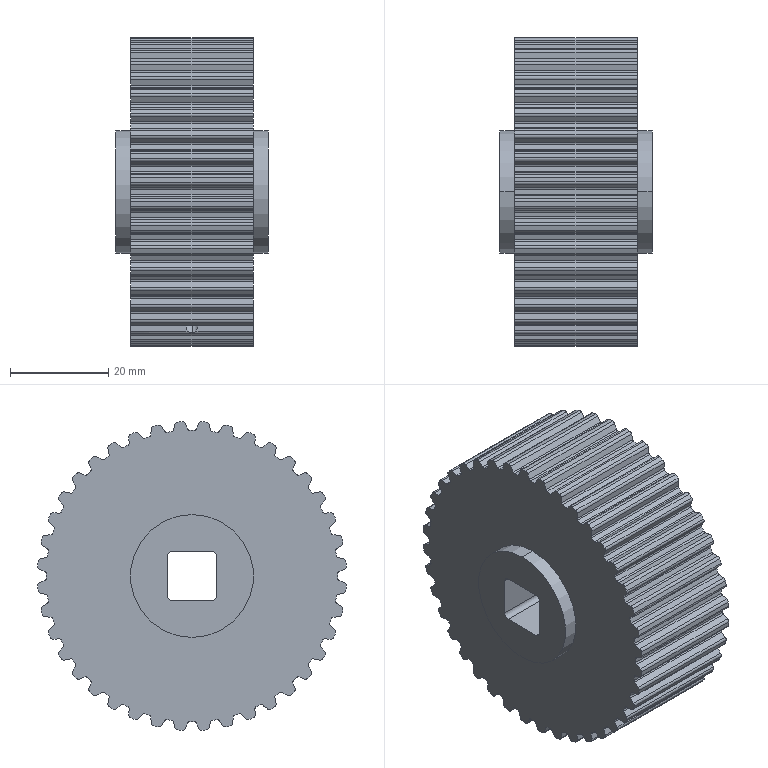Part | STEP file | TTPP40T5250-A-P11_b traction belt pulley | 1 solid | 352 faces | box 31 x 62.727 x 62.727 mm | volume 72805 mm3 | cylinder 260 | plane 92 | commonest cylinder face diameters 0.8 x84 1.2 x80 59.25 x42 62.85 x40 2 x4 3.242 x4